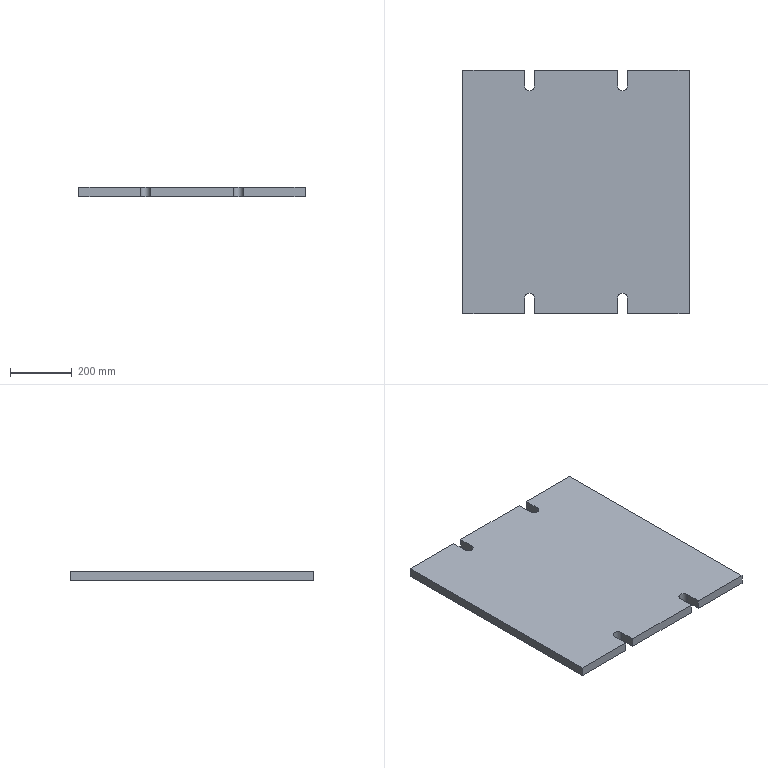Part | STEP file | 1 solid | 22 faces | box 730 x 785 x 30 mm | volume 16951245 mm3 | plane 18 | cylinder 4 | commonest cylinder face diameters 32 x4
STEP:
#1=CARTESIAN_POINT('',(129.,392.5,215.));
#2=VERTEX_POINT('',#1);
#3=CARTESIAN_POINT('',(-139.,392.5,215.));
#4=VERTEX_POINT('',#3);
#5=CARTESIAN_POINT('',(575.,392.5,215.));
#6=DIRECTION('',(-1.,0.,0.));
#7=VECTOR('',#6,1.);
#8=LINE('',#5,#7);
#9=EDGE_CURVE('',#2,#4,#8,.T.);
#10=ORIENTED_EDGE('',*,*,#9,.T.);
#11=CARTESIAN_POINT('',(-139.,392.5,245.));
#12=VERTEX_POINT('',#11);
#13=CARTESIAN_POINT('',(-139.,392.5,259.));
#14=DIRECTION('',(0.,0.,1.));
#15=VECTOR('',#14,1.);
#16=LINE('',#13,#15);
#17=EDGE_CURVE('',#4,#12,#16,.T.);
#18=ORIENTED_EDGE('',*,*,#17,.T.);
#19=CARTESIAN_POINT('',(129.,392.5,245.));
#20=VERTEX_POINT('',#19);
#21=CARTESIAN_POINT('',(575.,392.5,245.));
#22=DIRECTION('',(-1.,0.,0.));
#23=VECTOR('',#22,1.);
#24=LINE('',#21,#23);
#25=EDGE_CURVE('',#20,#12,#24,.T.);
#26=ORIENTED_EDGE('',*,*,#25,.F.);
#27=CARTESIAN_POINT('',(129.,392.5,259.));
#28=DIRECTION('',(0.,0.,-1.));
#29=VECTOR('',#28,1.);
#30=LINE('',#27,#29);
#31=EDGE_CURVE('',#20,#2,#30,.T.);
#32=ORIENTED_EDGE('',*,*,#31,.T.);
#33=EDGE_LOOP('',(#10,#18,#26,#32));
#34=FACE_OUTER_BOUND('',#33,.T.);
#35=CARTESIAN_POINT('',(575.,392.5,245.));
#36=DIRECTION('',(0.,-1.,0.));
#37=DIRECTION('',(0.,0.,-1.));
#38=AXIS2_PLACEMENT_3D('',#35,#36,#37);
#39=PLANE('',#38);
#40=ADVANCED_FACE('',(#34),#39,.F.);
#41=CARTESIAN_POINT('',(360.,392.5,215.));
#42=VERTEX_POINT('',#41);
#43=CARTESIAN_POINT('',(161.,392.5,215.));
#44=VERTEX_POINT('',#43);
#45=CARTESIAN_POINT('',(575.,392.5,215.));
#46=DIRECTION('',(-1.,0.,0.));
#47=VECTOR('',#46,1.);
#48=LINE('',#45,#47);
#49=EDGE_CURVE('',#42,#44,#48,.T.);
#50=ORIENTED_EDGE('',*,*,#49,.T.);
#51=CARTESIAN_POINT('',(161.,392.5,245.));
#52=VERTEX_POINT('',#51);
#53=CARTESIAN_POINT('',(161.,392.5,259.));
#54=DIRECTION('',(0.,0.,1.));
#55=VECTOR('',#54,1.);
#56=LINE('',#53,#55);
#57=EDGE_CURVE('',#44,#52,#56,.T.);
#58=ORIENTED_EDGE('',*,*,#57,.T.);
#59=CARTESIAN_POINT('',(360.,392.5,245.));
#60=VERTEX_POINT('',#59);
#61=CARTESIAN_POINT('',(575.,392.5,245.));
#62=DIRECTION('',(-1.,0.,0.));
#63=VECTOR('',#62,1.);
#64=LINE('',#61,#63);
#65=EDGE_CURVE('',#60,#52,#64,.T.);
#66=ORIENTED_EDGE('',*,*,#65,.F.);
#67=CARTESIAN_POINT('',(360.,392.5,245.));
#68=DIRECTION('',(0.,0.,-1.));
#69=VECTOR('',#68,1.);
#70=LINE('',#67,#69);
#71=EDGE_CURVE('',#60,#42,#70,.T.);
#72=ORIENTED_EDGE('',*,*,#71,.T.);
#73=EDGE_LOOP('',(#50,#58,#66,#72));
#74=FACE_OUTER_BOUND('',#73,.T.);
#75=CARTESIAN_POINT('',(575.,392.5,245.));
#76=DIRECTION('',(0.,-1.,0.));
#77=DIRECTION('',(0.,0.,-1.));
#78=AXIS2_PLACEMENT_3D('',#75,#76,#77);
#79=PLANE('',#78);
#80=ADVANCED_FACE('',(#74),#79,.F.);
#81=CARTESIAN_POINT('',(360.,-392.5,215.));
#82=VERTEX_POINT('',#81);
#83=CARTESIAN_POINT('',(360.,-267.5,215.));
#84=DIRECTION('',(0.,1.,0.));
#85=VECTOR('',#84,1.);
#86=LINE('',#83,#85);
#87=EDGE_CURVE('',#82,#42,#86,.T.);
#88=ORIENTED_EDGE('',*,*,#87,.T.);
#89=ORIENTED_EDGE('',*,*,#71,.F.);
#90=CARTESIAN_POINT('',(360.,-392.5,245.));
#91=VERTEX_POINT('',#90);
#92=CARTESIAN_POINT('',(360.,-267.5,245.));
#93=DIRECTION('',(0.,1.,0.));
#94=VECTOR('',#93,1.);
#95=LINE('',#92,#94);
#96=EDGE_CURVE('',#91,#60,#95,.T.);
#97=ORIENTED_EDGE('',*,*,#96,.F.);
#98=CARTESIAN_POINT('',(360.,-392.5,105.));
#99=DIRECTION('',(0.,0.,-1.));
#100=VECTOR('',#99,1.);
#101=LINE('',#98,#100);
#102=EDGE_CURVE('',#91,#82,#101,.T.);
#103=ORIENTED_EDGE('',*,*,#102,.T.);
#104=EDGE_LOOP('',(#88,#89,#97,#103));
#105=FACE_OUTER_BOUND('',#104,.T.);
#106=CARTESIAN_POINT('',(360.,-267.5,105.));
#107=DIRECTION('',(-1.,0.,0.));
#108=DIRECTION('',(0.,1.,0.));
#109=AXIS2_PLACEMENT_3D('',#106,#107,#108);
#110=PLANE('',#109);
#111=ADVANCED_FACE('',(#105),#110,.F.);
#112=CARTESIAN_POINT('',(161.,-392.5,245.));
#113=VERTEX_POINT('',#112);
#114=CARTESIAN_POINT('',(-585.,-392.5,245.));
#115=DIRECTION('',(1.,0.,0.));
#116=VECTOR('',#115,1.);
#117=LINE('',#114,#116);
#118=EDGE_CURVE('',#113,#91,#117,.T.);
#119=ORIENTED_EDGE('',*,*,#118,.F.);
#120=CARTESIAN_POINT('',(161.,-392.5,215.));
#121=VERTEX_POINT('',#120);
#122=CARTESIAN_POINT('',(161.,-392.5,259.));
#123=DIRECTION('',(0.,0.,-1.));
#124=VECTOR('',#123,1.);
#125=LINE('',#122,#124);
#126=EDGE_CURVE('',#113,#121,#125,.T.);
#127=ORIENTED_EDGE('',*,*,#126,.T.);
#128=CARTESIAN_POINT('',(-585.,-392.5,215.));
#129=DIRECTION('',(1.,0.,0.));
#130=VECTOR('',#129,1.);
#131=LINE('',#128,#130);
#132=EDGE_CURVE('',#121,#82,#131,.T.);
#133=ORIENTED_EDGE('',*,*,#132,.T.);
#134=ORIENTED_EDGE('',*,*,#102,.F.);
#135=EDGE_LOOP('',(#119,#127,#133,#134));
#136=FACE_OUTER_BOUND('',#135,.T.);
#137=CARTESIAN_POINT('',(-585.,-392.5,245.));
#138=DIRECTION('',(0.,1.,0.));
#139=DIRECTION('',(-1.,0.,0.));
#140=AXIS2_PLACEMENT_3D('',#137,#138,#139);
#141=PLANE('',#140);
#142=ADVANCED_FACE('',(#136),#141,.F.);
#143=ORIENTED_EDGE('',*,*,#126,.F.);
#144=CARTESIAN_POINT('',(161.,-342.5,245.));
#145=VERTEX_POINT('',#144);
#146=CARTESIAN_POINT('',(161.,-392.5,245.));
#147=DIRECTION('',(0.,-1.,0.));
#148=VECTOR('',#147,1.);
#149=LINE('',#146,#148);
#150=EDGE_CURVE('',#145,#113,#149,.T.);
#151=ORIENTED_EDGE('',*,*,#150,.F.);
#152=CARTESIAN_POINT('',(161.,-342.5,215.));
#153=VERTEX_POINT('',#152);
#154=CARTESIAN_POINT('',(161.,-342.5,259.));
#155=DIRECTION('',(0.,0.,1.));
#156=VECTOR('',#155,1.);
#157=LINE('',#154,#156);
#158=EDGE_CURVE('',#153,#145,#157,.T.);
#159=ORIENTED_EDGE('',*,*,#158,.F.);
#160=CARTESIAN_POINT('',(161.,-392.5,215.));
#161=DIRECTION('',(0.,1.,0.));
#162=VECTOR('',#161,1.);
#163=LINE('',#160,#162);
#164=EDGE_CURVE('',#121,#153,#163,.T.);
#165=ORIENTED_EDGE('',*,*,#164,.F.);
#166=EDGE_LOOP('',(#143,#151,#159,#165));
#167=FACE_OUTER_BOUND('',#166,.T.);
#168=CARTESIAN_POINT('',(161.,-392.5,259.));
#169=DIRECTION('',(1.,0.,0.));
#170=DIRECTION('',(0.,0.,1.));
#171=AXIS2_PLACEMENT_3D('',#168,#169,#170);
#172=PLANE('',#171);
#173=ADVANCED_FACE('',(#167),#172,.F.);
#174=ORIENTED_EDGE('',*,*,#158,.T.);
#175=CARTESIAN_POINT('',(129.,-342.5,245.));
#176=VERTEX_POINT('',#175);
#177=CARTESIAN_POINT('',(145.,-342.5,245.));
#178=DIRECTION('',(0.,0.,1.));
#179=DIRECTION('',(1.,0.,0.));
#180=AXIS2_PLACEMENT_3D('',#177,#178,#179);
#181=CIRCLE('',#180,16.);
#182=EDGE_CURVE('',#145,#176,#181,.T.);
#183=ORIENTED_EDGE('',*,*,#182,.T.);
#184=CARTESIAN_POINT('',(129.,-342.5,215.));
#185=VERTEX_POINT('',#184);
#186=CARTESIAN_POINT('',(129.,-342.5,259.));
#187=DIRECTION('',(0.,0.,1.));
#188=VECTOR('',#187,1.);
#189=LINE('',#186,#188);
#190=EDGE_CURVE('',#185,#176,#189,.T.);
#191=ORIENTED_EDGE('',*,*,#190,.F.);
#192=CARTESIAN_POINT('',(145.,-342.5,215.));
#193=DIRECTION('',(0.,0.,1.));
#194=DIRECTION('',(1.,0.,0.));
#195=AXIS2_PLACEMENT_3D('',#192,#193,#194);
#196=CIRCLE('',#195,16.);
#197=EDGE_CURVE('',#153,#185,#196,.T.);
#198=ORIENTED_EDGE('',*,*,#197,.F.);
#199=EDGE_LOOP('',(#174,#183,#191,#198));
#200=FACE_OUTER_BOUND('',#199,.T.);
#201=CARTESIAN_POINT('',(145.,-342.5,259.));
#202=DIRECTION('',(0.,0.,-1.));
#203=DIRECTION('',(1.,0.,0.));
#204=AXIS2_PLACEMENT_3D('',#201,#202,#203);
#205=CYLINDRICAL_SURFACE('',#204,16.);
#206=ADVANCED_FACE('',(#200),#205,.F.);
#207=ORIENTED_EDGE('',*,*,#190,.T.);
#208=CARTESIAN_POINT('',(129.,-392.5,245.));
#209=VERTEX_POINT('',#208);
#210=CARTESIAN_POINT('',(129.,-342.5,245.));
#211=DIRECTION('',(0.,1.,0.));
#212=VECTOR('',#211,1.);
#213=LINE('',#210,#212);
#214=EDGE_CURVE('',#209,#176,#213,.T.);
#215=ORIENTED_EDGE('',*,*,#214,.F.);
#216=CARTESIAN_POINT('',(129.,-392.5,215.));
#217=VERTEX_POINT('',#216);
#218=CARTESIAN_POINT('',(129.,-392.5,259.));
#219=DIRECTION('',(0.,0.,1.));
#220=VECTOR('',#219,1.);
#221=LINE('',#218,#220);
#222=EDGE_CURVE('',#217,#209,#221,.T.);
#223=ORIENTED_EDGE('',*,*,#222,.F.);
#224=CARTESIAN_POINT('',(129.,-342.5,215.));
#225=DIRECTION('',(0.,-1.,0.));
#226=VECTOR('',#225,1.);
#227=LINE('',#224,#226);
#228=EDGE_CURVE('',#185,#217,#227,.T.);
#229=ORIENTED_EDGE('',*,*,#228,.F.);
#230=EDGE_LOOP('',(#207,#215,#223,#229));
#231=FACE_OUTER_BOUND('',#230,.T.);
#232=CARTESIAN_POINT('',(129.,-342.5,259.));
#233=DIRECTION('',(-1.,0.,0.));
#234=DIRECTION('',(0.,0.,-1.));
#235=AXIS2_PLACEMENT_3D('',#232,#233,#234);
#236=PLANE('',#235);
#237=ADVANCED_FACE('',(#231),#236,.F.);
#238=CARTESIAN_POINT('',(-139.,-392.5,215.));
#239=VERTEX_POINT('',#238);
#240=CARTESIAN_POINT('',(-585.,-392.5,215.));
#241=DIRECTION('',(1.,0.,0.));
#242=VECTOR('',#241,1.);
#243=LINE('',#240,#242);
#244=EDGE_CURVE('',#239,#217,#243,.T.);
#245=ORIENTED_EDGE('',*,*,#244,.T.);
#246=ORIENTED_EDGE('',*,*,#222,.T.);
#247=CARTESIAN_POINT('',(-139.,-392.5,245.));
#248=VERTEX_POINT('',#247);
#249=CARTESIAN_POINT('',(-585.,-392.5,245.));
#250=DIRECTION('',(1.,0.,0.));
#251=VECTOR('',#250,1.);
#252=LINE('',#249,#251);
#253=EDGE_CURVE('',#248,#209,#252,.T.);
#254=ORIENTED_EDGE('',*,*,#253,.F.);
#255=CARTESIAN_POINT('',(-139.,-392.5,259.));
#256=DIRECTION('',(0.,0.,-1.));
#257=VECTOR('',#256,1.);
#258=LINE('',#255,#257);
#259=EDGE_CURVE('',#248,#239,#258,.T.);
#260=ORIENTED_EDGE('',*,*,#259,.T.);
#261=EDGE_LOOP('',(#245,#246,#254,#260));
#262=FACE_OUTER_BOUND('',#261,.T.);
#263=CARTESIAN_POINT('',(-585.,-392.5,245.));
#264=DIRECTION('',(0.,1.,0.));
#265=DIRECTION('',(-1.,0.,0.));
#266=AXIS2_PLACEMENT_3D('',#263,#264,#265);
#267=PLANE('',#266);
#268=ADVANCED_FACE('',(#262),#267,.F.);
#269=CARTESIAN_POINT('',(-139.,-342.5,245.));
#270=VERTEX_POINT('',#269);
#271=CARTESIAN_POINT('',(-139.,-342.5,215.));
#272=VERTEX_POINT('',#271);
#273=CARTESIAN_POINT('',(-139.,-342.5,259.));
#274=DIRECTION('',(0.,0.,-1.));
#275=VECTOR('',#274,1.);
#276=LINE('',#273,#275);
#277=EDGE_CURVE('',#270,#272,#276,.T.);
#278=ORIENTED_EDGE('',*,*,#277,.T.);
#279=CARTESIAN_POINT('',(-139.,-342.5,215.));
#280=DIRECTION('',(0.,1.,0.));
#281=VECTOR('',#280,1.);
#282=LINE('',#279,#281);
#283=EDGE_CURVE('',#239,#272,#282,.T.);
#284=ORIENTED_EDGE('',*,*,#283,.F.);
#285=ORIENTED_EDGE('',*,*,#259,.F.);
#286=CARTESIAN_POINT('',(-139.,-342.5,245.));
#287=DIRECTION('',(0.,-1.,0.));
#288=VECTOR('',#287,1.);
#289=LINE('',#286,#288);
#290=EDGE_CURVE('',#270,#248,#289,.T.);
#291=ORIENTED_EDGE('',*,*,#290,.F.);
#292=EDGE_LOOP('',(#278,#284,#285,#291));
#293=FACE_OUTER_BOUND('',#292,.T.);
#294=CARTESIAN_POINT('',(-139.,-342.5,259.));
#295=DIRECTION('',(1.,0.,0.));
#296=DIRECTION('',(0.,0.,-1.));
#297=AXIS2_PLACEMENT_3D('',#294,#295,#296);
#298=PLANE('',#297);
#299=ADVANCED_FACE('',(#293),#298,.F.);
#300=CARTESIAN_POINT('',(-171.,-342.5,245.));
#301=VERTEX_POINT('',#300);
#302=CARTESIAN_POINT('',(-171.,-342.5,215.));
#303=VERTEX_POINT('',#302);
#304=CARTESIAN_POINT('',(-171.,-342.5,259.));
#305=DIRECTION('',(0.,0.,-1.));
#306=VECTOR('',#305,1.);
#307=LINE('',#304,#306);
#308=EDGE_CURVE('',#301,#303,#307,.T.);
#309=ORIENTED_EDGE('',*,*,#308,.T.);
#310=CARTESIAN_POINT('',(-155.,-342.5,215.));
#311=DIRECTION('',(0.,0.,1.));
#312=DIRECTION('',(1.,0.,0.));
#313=AXIS2_PLACEMENT_3D('',#310,#311,#312);
#314=CIRCLE('',#313,16.);
#315=EDGE_CURVE('',#272,#303,#314,.T.);
#316=ORIENTED_EDGE('',*,*,#315,.F.);
#317=ORIENTED_EDGE('',*,*,#277,.F.);
#318=CARTESIAN_POINT('',(-155.,-342.5,245.));
#319=DIRECTION('',(0.,0.,-1.));
#320=DIRECTION('',(1.,0.,0.));
#321=AXIS2_PLACEMENT_3D('',#318,#319,#320);
#322=CIRCLE('',#321,16.);
#323=EDGE_CURVE('',#301,#270,#322,.T.);
#324=ORIENTED_EDGE('',*,*,#323,.F.);
#325=EDGE_LOOP('',(#309,#316,#317,#324));
#326=FACE_OUTER_BOUND('',#325,.T.);
#327=CARTESIAN_POINT('',(-155.,-342.5,259.));
#328=DIRECTION('',(0.,0.,-1.));
#329=DIRECTION('',(-1.,0.,0.));
#330=AXIS2_PLACEMENT_3D('',#327,#328,#329);
#331=CYLINDRICAL_SURFACE('',#330,16.);
#332=ADVANCED_FACE('',(#326),#331,.F.);
#333=CARTESIAN_POINT('',(-171.,-392.5,215.));
#334=VERTEX_POINT('',#333);
#335=CARTESIAN_POINT('',(-171.,-392.5,245.));
#336=VERTEX_POINT('',#335);
#337=CARTESIAN_POINT('',(-171.,-392.5,259.));
#338=DIRECTION('',(0.,0.,1.));
#339=VECTOR('',#338,1.);
#340=LINE('',#337,#339);
#341=EDGE_CURVE('',#334,#336,#340,.T.);
#342=ORIENTED_EDGE('',*,*,#341,.F.);
#343=CARTESIAN_POINT('',(-171.,-392.5,215.));
#344=DIRECTION('',(0.,-1.,0.));
#345=VECTOR('',#344,1.);
#346=LINE('',#343,#345);
#347=EDGE_CURVE('',#303,#334,#346,.T.);
#348=ORIENTED_EDGE('',*,*,#347,.F.);
#349=ORIENTED_EDGE('',*,*,#308,.F.);
#350=CARTESIAN_POINT('',(-171.,-392.5,245.));
#351=DIRECTION('',(0.,1.,0.));
#352=VECTOR('',#351,1.);
#353=LINE('',#350,#352);
#354=EDGE_CURVE('',#336,#301,#353,.T.);
#355=ORIENTED_EDGE('',*,*,#354,.F.);
#356=EDGE_LOOP('',(#342,#348,#349,#355));
#357=FACE_OUTER_BOUND('',#356,.T.);
#358=CARTESIAN_POINT('',(-171.,-392.5,259.));
#359=DIRECTION('',(-1.,0.,0.));
#360=DIRECTION('',(0.,0.,1.));
#361=AXIS2_PLACEMENT_3D('',#358,#359,#360);
#362=PLANE('',#361);
#363=ADVANCED_FACE('',(#357),#362,.F.);
#364=CARTESIAN_POINT('',(-370.,-392.5,215.));
#365=VERTEX_POINT('',#364);
#366=CARTESIAN_POINT('',(-585.,-392.5,215.));
#367=DIRECTION('',(1.,0.,0.));
#368=VECTOR('',#367,1.);
#369=LINE('',#366,#368);
#370=EDGE_CURVE('',#365,#334,#369,.T.);
#371=ORIENTED_EDGE('',*,*,#370,.T.);
#372=ORIENTED_EDGE('',*,*,#341,.T.);
#373=CARTESIAN_POINT('',(-370.,-392.5,245.));
#374=VERTEX_POINT('',#373);
#375=CARTESIAN_POINT('',(-585.,-392.5,245.));
#376=DIRECTION('',(1.,0.,0.));
#377=VECTOR('',#376,1.);
#378=LINE('',#375,#377);
#379=EDGE_CURVE('',#374,#336,#378,.T.);
#380=ORIENTED_EDGE('',*,*,#379,.F.);
#381=CARTESIAN_POINT('',(-370.,-392.5,245.));
#382=DIRECTION('',(0.,0.,-1.));
#383=VECTOR('',#382,1.);
#384=LINE('',#381,#383);
#385=EDGE_CURVE('',#374,#365,#384,.T.);
#386=ORIENTED_EDGE('',*,*,#385,.T.);
#387=EDGE_LOOP('',(#371,#372,#380,#386));
#388=FACE_OUTER_BOUND('',#387,.T.);
#389=CARTESIAN_POINT('',(-585.,-392.5,245.));
#390=DIRECTION('',(0.,1.,0.));
#391=DIRECTION('',(-1.,0.,0.));
#392=AXIS2_PLACEMENT_3D('',#389,#390,#391);
#393=PLANE('',#392);
#394=ADVANCED_FACE('',(#388),#393,.F.);
#395=CARTESIAN_POINT('',(-370.,392.5,215.));
#396=VERTEX_POINT('',#395);
#397=CARTESIAN_POINT('',(-370.,-127.4,215.));
#398=DIRECTION('',(0.,-1.,0.));
#399=VECTOR('',#398,1.);
#400=LINE('',#397,#399);
#401=EDGE_CURVE('',#396,#365,#400,.T.);
#402=ORIENTED_EDGE('',*,*,#401,.T.);
#403=ORIENTED_EDGE('',*,*,#385,.F.);
#404=CARTESIAN_POINT('',(-370.,392.5,245.));
#405=VERTEX_POINT('',#404);
#406=CARTESIAN_POINT('',(-370.,-127.4,245.));
#407=DIRECTION('',(0.,-1.,0.));
#408=VECTOR('',#407,1.);
#409=LINE('',#406,#408);
#410=EDGE_CURVE('',#405,#374,#409,.T.);
#411=ORIENTED_EDGE('',*,*,#410,.F.);
#412=CARTESIAN_POINT('',(-370.,392.5,138.004));
#413=DIRECTION('',(0.,0.,-1.));
#414=VECTOR('',#413,1.);
#415=LINE('',#412,#414);
#416=EDGE_CURVE('',#405,#396,#415,.T.);
#417=ORIENTED_EDGE('',*,*,#416,.T.);
#418=EDGE_LOOP('',(#402,#403,#411,#417));
#419=FACE_OUTER_BOUND('',#418,.T.);
#420=CARTESIAN_POINT('',(-370.,-127.4,138.004));
#421=DIRECTION('',(-1.,0.,0.));
#422=DIRECTION('',(0.,0.,-1.));
#423=AXIS2_PLACEMENT_3D('',#420,#421,#422);
#424=PLANE('',#423);
#425=ADVANCED_FACE('',(#419),#424,.T.);
#426=CARTESIAN_POINT('',(-171.,392.5,245.));
#427=VERTEX_POINT('',#426);
#428=CARTESIAN_POINT('',(575.,392.5,245.));
#429=DIRECTION('',(-1.,0.,0.));
#430=VECTOR('',#429,1.);
#431=LINE('',#428,#430);
#432=EDGE_CURVE('',#427,#405,#431,.T.);
#433=ORIENTED_EDGE('',*,*,#432,.F.);
#434=CARTESIAN_POINT('',(-171.,392.5,215.));
#435=VERTEX_POINT('',#434);
#436=CARTESIAN_POINT('',(-171.,392.5,259.));
#437=DIRECTION('',(0.,0.,-1.));
#438=VECTOR('',#437,1.);
#439=LINE('',#436,#438);
#440=EDGE_CURVE('',#427,#435,#439,.T.);
#441=ORIENTED_EDGE('',*,*,#440,.T.);
#442=CARTESIAN_POINT('',(575.,392.5,215.));
#443=DIRECTION('',(-1.,0.,0.));
#444=VECTOR('',#443,1.);
#445=LINE('',#442,#444);
#446=EDGE_CURVE('',#435,#396,#445,.T.);
#447=ORIENTED_EDGE('',*,*,#446,.T.);
#448=ORIENTED_EDGE('',*,*,#416,.F.);
#449=EDGE_LOOP('',(#433,#441,#447,#448));
#450=FACE_OUTER_BOUND('',#449,.T.);
#451=CARTESIAN_POINT('',(575.,392.5,245.));
#452=DIRECTION('',(0.,-1.,0.));
#453=DIRECTION('',(0.,0.,-1.));
#454=AXIS2_PLACEMENT_3D('',#451,#452,#453);
#455=PLANE('',#454);
#456=ADVANCED_FACE('',(#450),#455,.F.);
#457=CARTESIAN_POINT('',(-171.,342.5,245.));
#458=VERTEX_POINT('',#457);
#459=CARTESIAN_POINT('',(-139.,342.5,245.));
#460=VERTEX_POINT('',#459);
#461=CARTESIAN_POINT('',(-155.,342.5,245.));
#462=DIRECTION('',(0.,0.,1.));
#463=DIRECTION('',(1.,0.,0.));
#464=AXIS2_PLACEMENT_3D('',#461,#462,#463);
#465=CIRCLE('',#464,16.);
#466=EDGE_CURVE('',#458,#460,#465,.T.);
#467=ORIENTED_EDGE('',*,*,#466,.F.);
#468=CARTESIAN_POINT('',(-171.,392.5,245.));
#469=DIRECTION('',(0.,1.,0.));
#470=VECTOR('',#469,1.);
#471=LINE('',#468,#470);
#472=EDGE_CURVE('',#458,#427,#471,.T.);
#473=ORIENTED_EDGE('',*,*,#472,.T.);
#474=ORIENTED_EDGE('',*,*,#432,.T.);
#475=ORIENTED_EDGE('',*,*,#410,.T.);
#476=ORIENTED_EDGE('',*,*,#379,.T.);
#477=ORIENTED_EDGE('',*,*,#354,.T.);
#478=ORIENTED_EDGE('',*,*,#323,.T.);
#479=ORIENTED_EDGE('',*,*,#290,.T.);
#480=ORIENTED_EDGE('',*,*,#253,.T.);
#481=ORIENTED_EDGE('',*,*,#214,.T.);
#482=ORIENTED_EDGE('',*,*,#182,.F.);
#483=ORIENTED_EDGE('',*,*,#150,.T.);
#484=ORIENTED_EDGE('',*,*,#118,.T.);
#485=ORIENTED_EDGE('',*,*,#96,.T.);
#486=ORIENTED_EDGE('',*,*,#65,.T.);
#487=CARTESIAN_POINT('',(161.,342.5,245.));
#488=VERTEX_POINT('',#487);
#489=CARTESIAN_POINT('',(161.,392.5,245.));
#490=DIRECTION('',(0.,-1.,0.));
#491=VECTOR('',#490,1.);
#492=LINE('',#489,#491);
#493=EDGE_CURVE('',#52,#488,#492,.T.);
#494=ORIENTED_EDGE('',*,*,#493,.T.);
#495=CARTESIAN_POINT('',(129.,342.5,245.));
#496=VERTEX_POINT('',#495);
#497=CARTESIAN_POINT('',(145.,342.5,245.));
#498=DIRECTION('',(0.,0.,1.));
#499=DIRECTION('',(1.,0.,0.));
#500=AXIS2_PLACEMENT_3D('',#497,#498,#499);
#501=CIRCLE('',#500,16.);
#502=EDGE_CURVE('',#496,#488,#501,.T.);
#503=ORIENTED_EDGE('',*,*,#502,.F.);
#504=CARTESIAN_POINT('',(129.,342.5,245.));
#505=DIRECTION('',(0.,1.,0.));
#506=VECTOR('',#505,1.);
#507=LINE('',#504,#506);
#508=EDGE_CURVE('',#496,#20,#507,.T.);
#509=ORIENTED_EDGE('',*,*,#508,.T.);
#510=ORIENTED_EDGE('',*,*,#25,.T.);
#511=CARTESIAN_POINT('',(-139.,342.5,245.));
#512=DIRECTION('',(0.,-1.,0.));
#513=VECTOR('',#512,1.);
#514=LINE('',#511,#513);
#515=EDGE_CURVE('',#12,#460,#514,.T.);
#516=ORIENTED_EDGE('',*,*,#515,.T.);
#517=EDGE_LOOP('',(#467,#473,#474,#475,#476,#477,#478,#479,#480,#481,#482,#483,#484,#485,#486,#494,#503,#509,#510,#516));
#518=FACE_OUTER_BOUND('',#517,.T.);
#519=CARTESIAN_POINT('',(0.,0.,245.));
#520=DIRECTION('',(0.,0.,1.));
#521=DIRECTION('',(1.,0.,0.));
#522=AXIS2_PLACEMENT_3D('',#519,#520,#521);
#523=PLANE('',#522);
#524=ADVANCED_FACE('',(#518),#523,.T.);
#525=ORIENTED_EDGE('',*,*,#446,.F.);
#526=CARTESIAN_POINT('',(-171.,342.5,215.));
#527=VERTEX_POINT('',#526);
#528=CARTESIAN_POINT('',(-171.,392.5,215.));
#529=DIRECTION('',(0.,-1.,0.));
#530=VECTOR('',#529,1.);
#531=LINE('',#528,#530);
#532=EDGE_CURVE('',#435,#527,#531,.T.);
#533=ORIENTED_EDGE('',*,*,#532,.T.);
#534=CARTESIAN_POINT('',(-139.,342.5,215.));
#535=VERTEX_POINT('',#534);
#536=CARTESIAN_POINT('',(-155.,342.5,215.));
#537=DIRECTION('',(0.,0.,1.));
#538=DIRECTION('',(1.,0.,0.));
#539=AXIS2_PLACEMENT_3D('',#536,#537,#538);
#540=CIRCLE('',#539,16.);
#541=EDGE_CURVE('',#527,#535,#540,.T.);
#542=ORIENTED_EDGE('',*,*,#541,.T.);
#543=CARTESIAN_POINT('',(-139.,342.5,215.));
#544=DIRECTION('',(0.,1.,0.));
#545=VECTOR('',#544,1.);
#546=LINE('',#543,#545);
#547=EDGE_CURVE('',#535,#4,#546,.T.);
#548=ORIENTED_EDGE('',*,*,#547,.T.);
#549=ORIENTED_EDGE('',*,*,#9,.F.);
#550=CARTESIAN_POINT('',(129.,342.5,215.));
#551=VERTEX_POINT('',#550);
#552=CARTESIAN_POINT('',(129.,342.5,215.));
#553=DIRECTION('',(0.,-1.,0.));
#554=VECTOR('',#553,1.);
#555=LINE('',#552,#554);
#556=EDGE_CURVE('',#2,#551,#555,.T.);
#557=ORIENTED_EDGE('',*,*,#556,.T.);
#558=CARTESIAN_POINT('',(161.,342.5,215.));
#559=VERTEX_POINT('',#558);
#560=CARTESIAN_POINT('',(145.,342.5,215.));
#561=DIRECTION('',(0.,0.,1.));
#562=DIRECTION('',(1.,0.,0.));
#563=AXIS2_PLACEMENT_3D('',#560,#561,#562);
#564=CIRCLE('',#563,16.);
#565=EDGE_CURVE('',#551,#559,#564,.T.);
#566=ORIENTED_EDGE('',*,*,#565,.T.);
#567=CARTESIAN_POINT('',(161.,392.5,215.));
#568=DIRECTION('',(0.,1.,0.));
#569=VECTOR('',#568,1.);
#570=LINE('',#567,#569);
#571=EDGE_CURVE('',#559,#44,#570,.T.);
#572=ORIENTED_EDGE('',*,*,#571,.T.);
#573=ORIENTED_EDGE('',*,*,#49,.F.);
#574=ORIENTED_EDGE('',*,*,#87,.F.);
#575=ORIENTED_EDGE('',*,*,#132,.F.);
#576=ORIENTED_EDGE('',*,*,#164,.T.);
#577=ORIENTED_EDGE('',*,*,#197,.T.);
#578=ORIENTED_EDGE('',*,*,#228,.T.);
#579=ORIENTED_EDGE('',*,*,#244,.F.);
#580=ORIENTED_EDGE('',*,*,#283,.T.);
#581=ORIENTED_EDGE('',*,*,#315,.T.);
#582=ORIENTED_EDGE('',*,*,#347,.T.);
#583=ORIENTED_EDGE('',*,*,#370,.F.);
#584=ORIENTED_EDGE('',*,*,#401,.F.);
#585=EDGE_LOOP('',(#525,#533,#542,#548,#549,#557,#566,#572,#573,#574,#575,#576,#577,#578,#579,#580,#581,#582,#583,#584));
#586=FACE_OUTER_BOUND('',#585,.T.);
#587=CARTESIAN_POINT('',(0.,0.,215.));
#588=DIRECTION('',(0.,0.,1.));
#589=DIRECTION('',(1.,0.,0.));
#590=AXIS2_PLACEMENT_3D('',#587,#588,#589);
#591=PLANE('',#590);
#592=ADVANCED_FACE('',(#586),#591,.F.);
#593=CARTESIAN_POINT('',(129.,342.5,259.));
#594=DIRECTION('',(0.,0.,-1.));
#595=VECTOR('',#594,1.);
#596=LINE('',#593,#595);
#597=EDGE_CURVE('',#496,#551,#596,.T.);
#598=ORIENTED_EDGE('',*,*,#597,.T.);
#599=ORIENTED_EDGE('',*,*,#556,.F.);
#600=ORIENTED_EDGE('',*,*,#31,.F.);
#601=ORIENTED_EDGE('',*,*,#508,.F.);
#602=EDGE_LOOP('',(#598,#599,#600,#601));
#603=FACE_OUTER_BOUND('',#602,.T.);
#604=CARTESIAN_POINT('',(129.,342.5,259.));
#605=DIRECTION('',(-1.,0.,0.));
#606=DIRECTION('',(0.,0.,-1.));
#607=AXIS2_PLACEMENT_3D('',#604,#605,#606);
#608=PLANE('',#607);
#609=ADVANCED_FACE('',(#603),#608,.F.);
#610=ORIENTED_EDGE('',*,*,#57,.F.);
#611=ORIENTED_EDGE('',*,*,#571,.F.);
#612=CARTESIAN_POINT('',(161.,342.5,259.));
#613=DIRECTION('',(0.,0.,-1.));
#614=VECTOR('',#613,1.);
#615=LINE('',#612,#614);
#616=EDGE_CURVE('',#488,#559,#615,.T.);
#617=ORIENTED_EDGE('',*,*,#616,.F.);
#618=ORIENTED_EDGE('',*,*,#493,.F.);
#619=EDGE_LOOP('',(#610,#611,#617,#618));
#620=FACE_OUTER_BOUND('',#619,.T.);
#621=CARTESIAN_POINT('',(161.,392.5,259.));
#622=DIRECTION('',(1.,0.,0.));
#623=DIRECTION('',(0.,0.,1.));
#624=AXIS2_PLACEMENT_3D('',#621,#622,#623);
#625=PLANE('',#624);
#626=ADVANCED_FACE('',(#620),#625,.F.);
#627=ORIENTED_EDGE('',*,*,#616,.T.);
#628=ORIENTED_EDGE('',*,*,#565,.F.);
#629=ORIENTED_EDGE('',*,*,#597,.F.);
#630=ORIENTED_EDGE('',*,*,#502,.T.);
#631=EDGE_LOOP('',(#627,#628,#629,#630));
#632=FACE_OUTER_BOUND('',#631,.T.);
#633=CARTESIAN_POINT('',(145.,342.5,259.));
#634=DIRECTION('',(0.,0.,-1.));
#635=DIRECTION('',(1.,0.,0.));
#636=AXIS2_PLACEMENT_3D('',#633,#634,#635);
#637=CYLINDRICAL_SURFACE('',#636,16.);
#638=ADVANCED_FACE('',(#632),#637,.F.);
#639=CARTESIAN_POINT('',(-139.,342.5,259.));
#640=DIRECTION('',(0.,0.,1.));
#641=VECTOR('',#640,1.);
#642=LINE('',#639,#641);
#643=EDGE_CURVE('',#535,#460,#642,.T.);
#644=ORIENTED_EDGE('',*,*,#643,.T.);
#645=ORIENTED_EDGE('',*,*,#515,.F.);
#646=ORIENTED_EDGE('',*,*,#17,.F.);
#647=ORIENTED_EDGE('',*,*,#547,.F.);
#648=EDGE_LOOP('',(#644,#645,#646,#647));
#649=FACE_OUTER_BOUND('',#648,.T.);
#650=CARTESIAN_POINT('',(-139.,342.5,259.));
#651=DIRECTION('',(1.,0.,0.));
#652=DIRECTION('',(0.,0.,-1.));
#653=AXIS2_PLACEMENT_3D('',#650,#651,#652);
#654=PLANE('',#653);
#655=ADVANCED_FACE('',(#649),#654,.F.);
#656=ORIENTED_EDGE('',*,*,#440,.F.);
#657=ORIENTED_EDGE('',*,*,#472,.F.);
#658=CARTESIAN_POINT('',(-171.,342.5,259.));
#659=DIRECTION('',(0.,0.,1.));
#660=VECTOR('',#659,1.);
#661=LINE('',#658,#660);
#662=EDGE_CURVE('',#527,#458,#661,.T.);
#663=ORIENTED_EDGE('',*,*,#662,.F.);
#664=ORIENTED_EDGE('',*,*,#532,.F.);
#665=EDGE_LOOP('',(#656,#657,#663,#664));
#666=FACE_OUTER_BOUND('',#665,.T.);
#667=CARTESIAN_POINT('',(-171.,392.5,259.));
#668=DIRECTION('',(-1.,0.,0.));
#669=DIRECTION('',(0.,0.,1.));
#670=AXIS2_PLACEMENT_3D('',#667,#668,#669);
#671=PLANE('',#670);
#672=ADVANCED_FACE('',(#666),#671,.F.);
#673=ORIENTED_EDGE('',*,*,#662,.T.);
#674=ORIENTED_EDGE('',*,*,#466,.T.);
#675=ORIENTED_EDGE('',*,*,#643,.F.);
#676=ORIENTED_EDGE('',*,*,#541,.F.);
#677=EDGE_LOOP('',(#673,#674,#675,#676));
#678=FACE_OUTER_BOUND('',#677,.T.);
#679=CARTESIAN_POINT('',(-155.,342.5,259.));
#680=DIRECTION('',(0.,0.,-1.));
#681=DIRECTION('',(-1.,0.,0.));
#682=AXIS2_PLACEMENT_3D('',#679,#680,#681);
#683=CYLINDRICAL_SURFACE('',#682,16.);
#684=ADVANCED_FACE('',(#678),#683,.F.);
#685=CLOSED_SHELL('',(#40,#80,#111,#142,#173,#206,#237,#268,#299,#332,#363,#394,#425,#456,#524,#592,#609,#626,#638,#655,#672,#684));
#686=MANIFOLD_SOLID_BREP('',#685);
#687=(LENGTH_UNIT()NAMED_UNIT(*)SI_UNIT(.MILLI.,.METRE.));
#688=UNCERTAINTY_MEASURE_WITH_UNIT(LENGTH_MEASURE(0.00002),#687,'','');
#689=(NAMED_UNIT(*)PLANE_ANGLE_UNIT()SI_UNIT($,.RADIAN.));
#690=PLANE_ANGLE_MEASURE_WITH_UNIT(PLANE_ANGLE_MEASURE(0.01745),#689);
#691=DIMENSIONAL_EXPONENTS(0.,0.,0.,0.,0.,0.,0.);
#692=(CONVERSION_BASED_UNIT('DEGREE',#690)NAMED_UNIT(#691)PLANE_ANGLE_UNIT());
#693=(NAMED_UNIT(*)SI_UNIT($,.STERADIAN.)SOLID_ANGLE_UNIT());
#694=(GEOMETRIC_REPRESENTATION_CONTEXT(3)GLOBAL_UNCERTAINTY_ASSIGNED_CONTEXT((#688))GLOBAL_UNIT_ASSIGNED_CONTEXT((#687,#692,#693))REPRESENTATION_CONTEXT('',''));
#695=ADVANCED_BREP_SHAPE_REPRESENTATION('',(#686),#694);